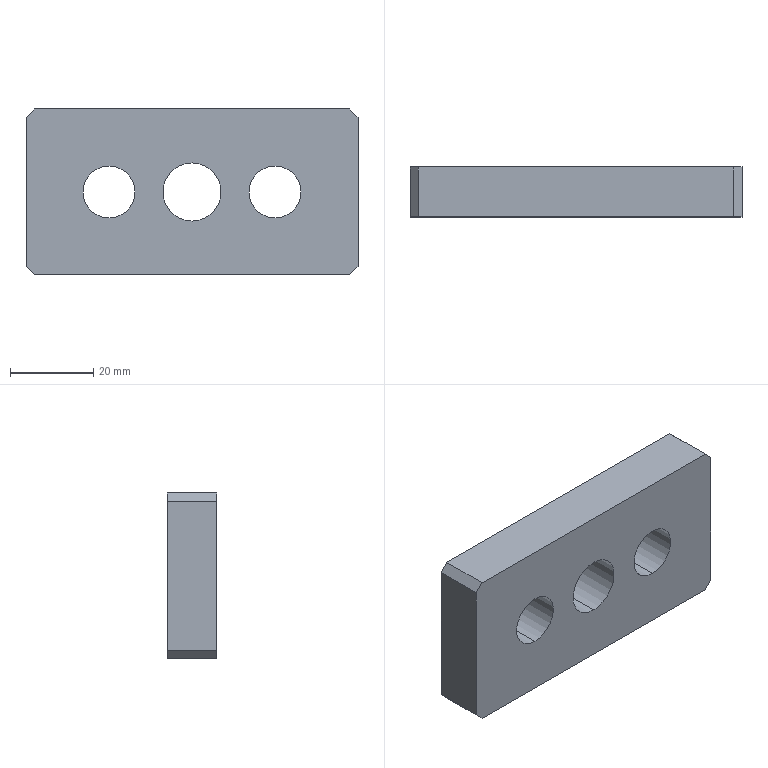Part | STEP file | PN_0026_default | 1 solid | 16 faces | box 80 x 12 x 40 mm | volume 33512 mm3 | plane 10 | cylinder 6 | commonest cylinder face diameters 12.5 x4 14 x2
STEP:
#1=CARTESIAN_POINT('',(0.,0.,0.));
#2=DIRECTION('',(0.,0.,1.));
#3=DIRECTION('',(1.,0.,0.));
#4=AXIS2_PLACEMENT_3D('',#1,#2,#3);
#5=CARTESIAN_POINT('',(-20.,12.,-6.25));
#6=VERTEX_POINT('',#5);
#7=CARTESIAN_POINT('',(-20.,0.,-6.25));
#8=VERTEX_POINT('',#7);
#9=CARTESIAN_POINT('',(-20.,0.,-6.25));
#10=DIRECTION('',(0.,-1.,0.));
#11=VECTOR('',#10,1.);
#12=LINE('',#9,#11);
#13=CARTESIAN_POINT('',(-20.,0.,0.));
#14=DIRECTION('',(0.,-1.,0.));
#15=DIRECTION('',(0.,0.,-1.));
#16=AXIS2_PLACEMENT_3D('',#13,#14,#15);
#17=CYLINDRICAL_SURFACE('',#16,6.25);
#18=CARTESIAN_POINT('',(6.283,0.));
#19=DIRECTION('',(0.,1.));
#20=VECTOR('',#19,1.);
#21=LINE('',#18,#20);
#22=(GEOMETRIC_REPRESENTATION_CONTEXT(2)PARAMETRIC_REPRESENTATION_CONTEXT()REPRESENTATION_CONTEXT('',''));
#23=DEFINITIONAL_REPRESENTATION('',(#21),#22);
#24=PCURVE('',#17,#23);
#25=CARTESIAN_POINT('',(-20.,0.,0.));
#26=DIRECTION('',(0.,-1.,0.));
#27=DIRECTION('',(0.,0.,-1.));
#28=AXIS2_PLACEMENT_3D('',#25,#26,#27);
#29=CYLINDRICAL_SURFACE('',#28,6.25);
#30=CARTESIAN_POINT('',(0.,0.));
#31=DIRECTION('',(0.,1.));
#32=VECTOR('',#31,1.);
#33=LINE('',#30,#32);
#34=(GEOMETRIC_REPRESENTATION_CONTEXT(2)PARAMETRIC_REPRESENTATION_CONTEXT()REPRESENTATION_CONTEXT('',''));
#35=DEFINITIONAL_REPRESENTATION('',(#33),#34);
#36=PCURVE('',#29,#35);
#37=SURFACE_CURVE('',#12,(#24,#36),.PCURVE_S1.);
#38=EDGE_CURVE('',#6,#8,#37,.T.);
#39=ORIENTED_EDGE('',*,*,#38,.T.);
#40=CARTESIAN_POINT('',(-20.,0.,6.25));
#41=VERTEX_POINT('',#40);
#42=CARTESIAN_POINT('',(-20.,0.,0.));
#43=DIRECTION('',(0.,-1.,0.));
#44=DIRECTION('',(0.,0.,-1.));
#45=AXIS2_PLACEMENT_3D('',#42,#43,#44);
#46=CIRCLE('',#45,6.25);
#47=CARTESIAN_POINT('',(0.,0.));
#48=DIRECTION('',(1.,0.));
#49=VECTOR('',#48,1.);
#50=LINE('',#47,#49);
#51=(GEOMETRIC_REPRESENTATION_CONTEXT(2)PARAMETRIC_REPRESENTATION_CONTEXT()REPRESENTATION_CONTEXT('',''));
#52=DEFINITIONAL_REPRESENTATION('',(#50),#51);
#53=PCURVE('',#17,#52);
#54=CARTESIAN_POINT('',(0.,0.,0.));
#55=DIRECTION('',(0.,1.,0.));
#56=DIRECTION('',(0.,0.,1.));
#57=AXIS2_PLACEMENT_3D('',#54,#55,#56);
#58=PLANE('',#57);
#59=CARTESIAN_POINT('',(-6.25,-20.));
#60=CARTESIAN_POINT('',(-6.25,-9.175));
#61=CARTESIAN_POINT('',(3.125,-14.587));
#62=CARTESIAN_POINT('',(12.5,-20.));
#63=CARTESIAN_POINT('',(3.125,-25.413));
#64=CARTESIAN_POINT('',(-6.25,-30.825));
#65=CARTESIAN_POINT('',(-6.25,-20.));
#66=(BOUNDED_CURVE()B_SPLINE_CURVE(2,(#59,#60,#61,#62,#63,#64,#65),.UNSPECIFIED.,.T.,.F.)B_SPLINE_CURVE_WITH_KNOTS((1,2,2,2,2,1),(-2.094,0.,2.094,4.189,6.283,8.378),.UNSPECIFIED.)CURVE()GEOMETRIC_REPRESENTATION_ITEM()RATIONAL_B_SPLINE_CURVE((1.,0.5,1.,0.5,1.,0.5,1.))REPRESENTATION_ITEM(''));
#67=(GEOMETRIC_REPRESENTATION_CONTEXT(2)PARAMETRIC_REPRESENTATION_CONTEXT()REPRESENTATION_CONTEXT('',''));
#68=DEFINITIONAL_REPRESENTATION('',(#66),#67);
#69=PCURVE('',#58,#68);
#70=SURFACE_CURVE('',#46,(#53,#69),.PCURVE_S1.);
#71=EDGE_CURVE('',#41,#8,#70,.T.);
#72=ORIENTED_EDGE('',*,*,#71,.F.);
#73=CARTESIAN_POINT('',(-20.,12.,6.25));
#74=VERTEX_POINT('',#73);
#75=CARTESIAN_POINT('',(-20.,0.,6.25));
#76=DIRECTION('',(0.,-1.,0.));
#77=VECTOR('',#76,1.);
#78=LINE('',#75,#77);
#79=CARTESIAN_POINT('',(3.142,0.));
#80=DIRECTION('',(0.,1.));
#81=VECTOR('',#80,1.);
#82=LINE('',#79,#81);
#83=(GEOMETRIC_REPRESENTATION_CONTEXT(2)PARAMETRIC_REPRESENTATION_CONTEXT()REPRESENTATION_CONTEXT('',''));
#84=DEFINITIONAL_REPRESENTATION('',(#82),#83);
#85=PCURVE('',#17,#84);
#86=CARTESIAN_POINT('',(3.142,0.));
#87=DIRECTION('',(0.,1.));
#88=VECTOR('',#87,1.);
#89=LINE('',#86,#88);
#90=(GEOMETRIC_REPRESENTATION_CONTEXT(2)PARAMETRIC_REPRESENTATION_CONTEXT()REPRESENTATION_CONTEXT('',''));
#91=DEFINITIONAL_REPRESENTATION('',(#89),#90);
#92=PCURVE('',#29,#91);
#93=SURFACE_CURVE('',#78,(#85,#92),.PCURVE_S1.);
#94=EDGE_CURVE('',#74,#41,#93,.T.);
#95=ORIENTED_EDGE('',*,*,#94,.F.);
#96=CARTESIAN_POINT('',(-20.,12.,0.));
#97=DIRECTION('',(0.,-1.,0.));
#98=DIRECTION('',(0.,0.,-1.));
#99=AXIS2_PLACEMENT_3D('',#96,#97,#98);
#100=CIRCLE('',#99,6.25);
#101=CARTESIAN_POINT('',(0.,-12.));
#102=DIRECTION('',(1.,0.));
#103=VECTOR('',#102,1.);
#104=LINE('',#101,#103);
#105=(GEOMETRIC_REPRESENTATION_CONTEXT(2)PARAMETRIC_REPRESENTATION_CONTEXT()REPRESENTATION_CONTEXT('',''));
#106=DEFINITIONAL_REPRESENTATION('',(#104),#105);
#107=PCURVE('',#17,#106);
#108=CARTESIAN_POINT('',(0.,12.,0.));
#109=DIRECTION('',(0.,1.,0.));
#110=DIRECTION('',(0.,0.,1.));
#111=AXIS2_PLACEMENT_3D('',#108,#109,#110);
#112=PLANE('',#111);
#113=CARTESIAN_POINT('',(-6.25,-20.));
#114=CARTESIAN_POINT('',(-6.25,-9.175));
#115=CARTESIAN_POINT('',(3.125,-14.587));
#116=CARTESIAN_POINT('',(12.5,-20.));
#117=CARTESIAN_POINT('',(3.125,-25.413));
#118=CARTESIAN_POINT('',(-6.25,-30.825));
#119=CARTESIAN_POINT('',(-6.25,-20.));
#120=(BOUNDED_CURVE()B_SPLINE_CURVE(2,(#113,#114,#115,#116,#117,#118,#119),.UNSPECIFIED.,.T.,.F.)B_SPLINE_CURVE_WITH_KNOTS((1,2,2,2,2,1),(-2.094,0.,2.094,4.189,6.283,8.378),.UNSPECIFIED.)CURVE()GEOMETRIC_REPRESENTATION_ITEM()RATIONAL_B_SPLINE_CURVE((1.,0.5,1.,0.5,1.,0.5,1.))REPRESENTATION_ITEM(''));
#121=(GEOMETRIC_REPRESENTATION_CONTEXT(2)PARAMETRIC_REPRESENTATION_CONTEXT()REPRESENTATION_CONTEXT('',''));
#122=DEFINITIONAL_REPRESENTATION('',(#120),#121);
#123=PCURVE('',#112,#122);
#124=SURFACE_CURVE('',#100,(#107,#123),.PCURVE_S1.);
#125=EDGE_CURVE('',#74,#6,#124,.T.);
#126=ORIENTED_EDGE('',*,*,#125,.T.);
#127=EDGE_LOOP('',(#39,#72,#95,#126));
#128=FACE_BOUND('',#127,.F.);
#129=ADVANCED_FACE('',(#128),#17,.F.);
#130=CARTESIAN_POINT('',(20.,12.,-6.25));
#131=VERTEX_POINT('',#130);
#132=CARTESIAN_POINT('',(20.,0.,-6.25));
#133=VERTEX_POINT('',#132);
#134=CARTESIAN_POINT('',(20.,0.,-6.25));
#135=DIRECTION('',(0.,-1.,0.));
#136=VECTOR('',#135,1.);
#137=LINE('',#134,#136);
#138=CARTESIAN_POINT('',(20.,0.,0.));
#139=DIRECTION('',(0.,-1.,0.));
#140=DIRECTION('',(0.,0.,-1.));
#141=AXIS2_PLACEMENT_3D('',#138,#139,#140);
#142=CYLINDRICAL_SURFACE('',#141,6.25);
#143=CARTESIAN_POINT('',(6.283,0.));
#144=DIRECTION('',(0.,1.));
#145=VECTOR('',#144,1.);
#146=LINE('',#143,#145);
#147=(GEOMETRIC_REPRESENTATION_CONTEXT(2)PARAMETRIC_REPRESENTATION_CONTEXT()REPRESENTATION_CONTEXT('',''));
#148=DEFINITIONAL_REPRESENTATION('',(#146),#147);
#149=PCURVE('',#142,#148);
#150=CARTESIAN_POINT('',(20.,0.,0.));
#151=DIRECTION('',(0.,-1.,0.));
#152=DIRECTION('',(0.,0.,-1.));
#153=AXIS2_PLACEMENT_3D('',#150,#151,#152);
#154=CYLINDRICAL_SURFACE('',#153,6.25);
#155=CARTESIAN_POINT('',(0.,0.));
#156=DIRECTION('',(0.,1.));
#157=VECTOR('',#156,1.);
#158=LINE('',#155,#157);
#159=(GEOMETRIC_REPRESENTATION_CONTEXT(2)PARAMETRIC_REPRESENTATION_CONTEXT()REPRESENTATION_CONTEXT('',''));
#160=DEFINITIONAL_REPRESENTATION('',(#158),#159);
#161=PCURVE('',#154,#160);
#162=SURFACE_CURVE('',#137,(#149,#161),.PCURVE_S1.);
#163=EDGE_CURVE('',#131,#133,#162,.T.);
#164=ORIENTED_EDGE('',*,*,#163,.T.);
#165=CARTESIAN_POINT('',(20.,0.,6.25));
#166=VERTEX_POINT('',#165);
#167=CARTESIAN_POINT('',(20.,0.,0.));
#168=DIRECTION('',(0.,-1.,0.));
#169=DIRECTION('',(0.,0.,-1.));
#170=AXIS2_PLACEMENT_3D('',#167,#168,#169);
#171=CIRCLE('',#170,6.25);
#172=CARTESIAN_POINT('',(0.,0.));
#173=DIRECTION('',(1.,0.));
#174=VECTOR('',#173,1.);
#175=LINE('',#172,#174);
#176=(GEOMETRIC_REPRESENTATION_CONTEXT(2)PARAMETRIC_REPRESENTATION_CONTEXT()REPRESENTATION_CONTEXT('',''));
#177=DEFINITIONAL_REPRESENTATION('',(#175),#176);
#178=PCURVE('',#142,#177);
#179=CARTESIAN_POINT('',(-6.25,20.));
#180=CARTESIAN_POINT('',(-6.25,30.825));
#181=CARTESIAN_POINT('',(3.125,25.413));
#182=CARTESIAN_POINT('',(12.5,20.));
#183=CARTESIAN_POINT('',(3.125,14.587));
#184=CARTESIAN_POINT('',(-6.25,9.175));
#185=CARTESIAN_POINT('',(-6.25,20.));
#186=(BOUNDED_CURVE()B_SPLINE_CURVE(2,(#179,#180,#181,#182,#183,#184,#185),.UNSPECIFIED.,.T.,.F.)B_SPLINE_CURVE_WITH_KNOTS((1,2,2,2,2,1),(-2.094,0.,2.094,4.189,6.283,8.378),.UNSPECIFIED.)CURVE()GEOMETRIC_REPRESENTATION_ITEM()RATIONAL_B_SPLINE_CURVE((1.,0.5,1.,0.5,1.,0.5,1.))REPRESENTATION_ITEM(''));
#187=(GEOMETRIC_REPRESENTATION_CONTEXT(2)PARAMETRIC_REPRESENTATION_CONTEXT()REPRESENTATION_CONTEXT('',''));
#188=DEFINITIONAL_REPRESENTATION('',(#186),#187);
#189=PCURVE('',#58,#188);
#190=SURFACE_CURVE('',#171,(#178,#189),.PCURVE_S1.);
#191=EDGE_CURVE('',#166,#133,#190,.T.);
#192=ORIENTED_EDGE('',*,*,#191,.F.);
#193=CARTESIAN_POINT('',(20.,12.,6.25));
#194=VERTEX_POINT('',#193);
#195=CARTESIAN_POINT('',(20.,0.,6.25));
#196=DIRECTION('',(0.,-1.,0.));
#197=VECTOR('',#196,1.);
#198=LINE('',#195,#197);
#199=CARTESIAN_POINT('',(3.142,0.));
#200=DIRECTION('',(0.,1.));
#201=VECTOR('',#200,1.);
#202=LINE('',#199,#201);
#203=(GEOMETRIC_REPRESENTATION_CONTEXT(2)PARAMETRIC_REPRESENTATION_CONTEXT()REPRESENTATION_CONTEXT('',''));
#204=DEFINITIONAL_REPRESENTATION('',(#202),#203);
#205=PCURVE('',#142,#204);
#206=CARTESIAN_POINT('',(3.142,0.));
#207=DIRECTION('',(0.,1.));
#208=VECTOR('',#207,1.);
#209=LINE('',#206,#208);
#210=(GEOMETRIC_REPRESENTATION_CONTEXT(2)PARAMETRIC_REPRESENTATION_CONTEXT()REPRESENTATION_CONTEXT('',''));
#211=DEFINITIONAL_REPRESENTATION('',(#209),#210);
#212=PCURVE('',#154,#211);
#213=SURFACE_CURVE('',#198,(#205,#212),.PCURVE_S1.);
#214=EDGE_CURVE('',#194,#166,#213,.T.);
#215=ORIENTED_EDGE('',*,*,#214,.F.);
#216=CARTESIAN_POINT('',(20.,12.,0.));
#217=DIRECTION('',(0.,-1.,0.));
#218=DIRECTION('',(0.,0.,-1.));
#219=AXIS2_PLACEMENT_3D('',#216,#217,#218);
#220=CIRCLE('',#219,6.25);
#221=CARTESIAN_POINT('',(0.,-12.));
#222=DIRECTION('',(1.,0.));
#223=VECTOR('',#222,1.);
#224=LINE('',#221,#223);
#225=(GEOMETRIC_REPRESENTATION_CONTEXT(2)PARAMETRIC_REPRESENTATION_CONTEXT()REPRESENTATION_CONTEXT('',''));
#226=DEFINITIONAL_REPRESENTATION('',(#224),#225);
#227=PCURVE('',#142,#226);
#228=CARTESIAN_POINT('',(-6.25,20.));
#229=CARTESIAN_POINT('',(-6.25,30.825));
#230=CARTESIAN_POINT('',(3.125,25.413));
#231=CARTESIAN_POINT('',(12.5,20.));
#232=CARTESIAN_POINT('',(3.125,14.587));
#233=CARTESIAN_POINT('',(-6.25,9.175));
#234=CARTESIAN_POINT('',(-6.25,20.));
#235=(BOUNDED_CURVE()B_SPLINE_CURVE(2,(#228,#229,#230,#231,#232,#233,#234),.UNSPECIFIED.,.T.,.F.)B_SPLINE_CURVE_WITH_KNOTS((1,2,2,2,2,1),(-2.094,0.,2.094,4.189,6.283,8.378),.UNSPECIFIED.)CURVE()GEOMETRIC_REPRESENTATION_ITEM()RATIONAL_B_SPLINE_CURVE((1.,0.5,1.,0.5,1.,0.5,1.))REPRESENTATION_ITEM(''));
#236=(GEOMETRIC_REPRESENTATION_CONTEXT(2)PARAMETRIC_REPRESENTATION_CONTEXT()REPRESENTATION_CONTEXT('',''));
#237=DEFINITIONAL_REPRESENTATION('',(#235),#236);
#238=PCURVE('',#112,#237);
#239=SURFACE_CURVE('',#220,(#227,#238),.PCURVE_S1.);
#240=EDGE_CURVE('',#194,#131,#239,.T.);
#241=ORIENTED_EDGE('',*,*,#240,.T.);
#242=EDGE_LOOP('',(#164,#192,#215,#241));
#243=FACE_BOUND('',#242,.F.);
#244=ADVANCED_FACE('',(#243),#142,.F.);
#245=CARTESIAN_POINT('',(0.,12.,-7.));
#246=VERTEX_POINT('',#245);
#247=CARTESIAN_POINT('',(0.,0.,-7.));
#248=VERTEX_POINT('',#247);
#249=CARTESIAN_POINT('',(0.,0.,-7.));
#250=DIRECTION('',(0.,-1.,0.));
#251=VECTOR('',#250,1.);
#252=LINE('',#249,#251);
#253=CARTESIAN_POINT('',(0.,0.,0.));
#254=DIRECTION('',(0.,-1.,0.));
#255=DIRECTION('',(0.,0.,-1.));
#256=AXIS2_PLACEMENT_3D('',#253,#254,#255);
#257=CYLINDRICAL_SURFACE('',#256,7.);
#258=CARTESIAN_POINT('',(6.283,0.));
#259=DIRECTION('',(0.,1.));
#260=VECTOR('',#259,1.);
#261=LINE('',#258,#260);
#262=(GEOMETRIC_REPRESENTATION_CONTEXT(2)PARAMETRIC_REPRESENTATION_CONTEXT()REPRESENTATION_CONTEXT('',''));
#263=DEFINITIONAL_REPRESENTATION('',(#261),#262);
#264=PCURVE('',#257,#263);
#265=CARTESIAN_POINT('',(0.,0.,0.));
#266=DIRECTION('',(0.,-1.,0.));
#267=DIRECTION('',(0.,0.,-1.));
#268=AXIS2_PLACEMENT_3D('',#265,#266,#267);
#269=CYLINDRICAL_SURFACE('',#268,7.);
#270=CARTESIAN_POINT('',(0.,0.));
#271=DIRECTION('',(0.,1.));
#272=VECTOR('',#271,1.);
#273=LINE('',#270,#272);
#274=(GEOMETRIC_REPRESENTATION_CONTEXT(2)PARAMETRIC_REPRESENTATION_CONTEXT()REPRESENTATION_CONTEXT('',''));
#275=DEFINITIONAL_REPRESENTATION('',(#273),#274);
#276=PCURVE('',#269,#275);
#277=SURFACE_CURVE('',#252,(#264,#276),.PCURVE_S1.);
#278=EDGE_CURVE('',#246,#248,#277,.T.);
#279=ORIENTED_EDGE('',*,*,#278,.T.);
#280=CARTESIAN_POINT('',(0.,0.,7.));
#281=VERTEX_POINT('',#280);
#282=CARTESIAN_POINT('',(0.,0.,0.));
#283=DIRECTION('',(0.,-1.,0.));
#284=DIRECTION('',(0.,0.,-1.));
#285=AXIS2_PLACEMENT_3D('',#282,#283,#284);
#286=CIRCLE('',#285,7.);
#287=CARTESIAN_POINT('',(0.,0.));
#288=DIRECTION('',(1.,0.));
#289=VECTOR('',#288,1.);
#290=LINE('',#287,#289);
#291=(GEOMETRIC_REPRESENTATION_CONTEXT(2)PARAMETRIC_REPRESENTATION_CONTEXT()REPRESENTATION_CONTEXT('',''));
#292=DEFINITIONAL_REPRESENTATION('',(#290),#291);
#293=PCURVE('',#257,#292);
#294=CARTESIAN_POINT('',(-7.,0.));
#295=CARTESIAN_POINT('',(-7.,12.124));
#296=CARTESIAN_POINT('',(3.5,6.062));
#297=CARTESIAN_POINT('',(14.,0.));
#298=CARTESIAN_POINT('',(3.5,-6.062));
#299=CARTESIAN_POINT('',(-7.,-12.124));
#300=CARTESIAN_POINT('',(-7.,0.));
#301=(BOUNDED_CURVE()B_SPLINE_CURVE(2,(#294,#295,#296,#297,#298,#299,#300),.UNSPECIFIED.,.T.,.F.)B_SPLINE_CURVE_WITH_KNOTS((1,2,2,2,2,1),(-2.094,0.,2.094,4.189,6.283,8.378),.UNSPECIFIED.)CURVE()GEOMETRIC_REPRESENTATION_ITEM()RATIONAL_B_SPLINE_CURVE((1.,0.5,1.,0.5,1.,0.5,1.))REPRESENTATION_ITEM(''));
#302=(GEOMETRIC_REPRESENTATION_CONTEXT(2)PARAMETRIC_REPRESENTATION_CONTEXT()REPRESENTATION_CONTEXT('',''));
#303=DEFINITIONAL_REPRESENTATION('',(#301),#302);
#304=PCURVE('',#58,#303);
#305=SURFACE_CURVE('',#286,(#293,#304),.PCURVE_S1.);
#306=EDGE_CURVE('',#281,#248,#305,.T.);
#307=ORIENTED_EDGE('',*,*,#306,.F.);
#308=CARTESIAN_POINT('',(0.,12.,7.));
#309=VERTEX_POINT('',#308);
#310=CARTESIAN_POINT('',(0.,0.,7.));
#311=DIRECTION('',(0.,-1.,0.));
#312=VECTOR('',#311,1.);
#313=LINE('',#310,#312);
#314=CARTESIAN_POINT('',(3.142,0.));
#315=DIRECTION('',(0.,1.));
#316=VECTOR('',#315,1.);
#317=LINE('',#314,#316);
#318=(GEOMETRIC_REPRESENTATION_CONTEXT(2)PARAMETRIC_REPRESENTATION_CONTEXT()REPRESENTATION_CONTEXT('',''));
#319=DEFINITIONAL_REPRESENTATION('',(#317),#318);
#320=PCURVE('',#257,#319);
#321=CARTESIAN_POINT('',(3.142,0.));
#322=DIRECTION('',(0.,1.));
#323=VECTOR('',#322,1.);
#324=LINE('',#321,#323);
#325=(GEOMETRIC_REPRESENTATION_CONTEXT(2)PARAMETRIC_REPRESENTATION_CONTEXT()REPRESENTATION_CONTEXT('',''));
#326=DEFINITIONAL_REPRESENTATION('',(#324),#325);
#327=PCURVE('',#269,#326);
#328=SURFACE_CURVE('',#313,(#320,#327),.PCURVE_S1.);
#329=EDGE_CURVE('',#309,#281,#328,.T.);
#330=ORIENTED_EDGE('',*,*,#329,.F.);
#331=CARTESIAN_POINT('',(0.,12.,0.));
#332=DIRECTION('',(0.,1.,0.));
#333=DIRECTION('',(0.,0.,1.));
#334=AXIS2_PLACEMENT_3D('',#331,#332,#333);
#335=CIRCLE('',#334,7.);
#336=CARTESIAN_POINT('',(9.425,-12.));
#337=DIRECTION('',(-1.,0.));
#338=VECTOR('',#337,1.);
#339=LINE('',#336,#338);
#340=(GEOMETRIC_REPRESENTATION_CONTEXT(2)PARAMETRIC_REPRESENTATION_CONTEXT()REPRESENTATION_CONTEXT('',''));
#341=DEFINITIONAL_REPRESENTATION('',(#339),#340);
#342=PCURVE('',#257,#341);
#343=CARTESIAN_POINT('',(0.,0.));
#344=DIRECTION('',(1.,0.));
#345=AXIS2_PLACEMENT_2D('',#343,#344);
#346=CIRCLE('',#345,7.);
#347=(GEOMETRIC_REPRESENTATION_CONTEXT(2)PARAMETRIC_REPRESENTATION_CONTEXT()REPRESENTATION_CONTEXT('',''));
#348=DEFINITIONAL_REPRESENTATION('',(#346),#347);
#349=PCURVE('',#112,#348);
#350=SURFACE_CURVE('',#335,(#342,#349),.PCURVE_S1.);
#351=EDGE_CURVE('',#246,#309,#350,.T.);
#352=ORIENTED_EDGE('',*,*,#351,.F.);
#353=EDGE_LOOP('',(#279,#307,#330,#352));
#354=FACE_BOUND('',#353,.F.);
#355=ADVANCED_FACE('',(#354),#257,.F.);
#356=CARTESIAN_POINT('',(40.,0.,18.));
#357=VERTEX_POINT('',#356);
#358=CARTESIAN_POINT('',(40.,0.,-18.));
#359=VERTEX_POINT('',#358);
#360=CARTESIAN_POINT('',(40.,0.,-20.));
#361=DIRECTION('',(0.,0.,-1.));
#362=VECTOR('',#361,1.);
#363=LINE('',#360,#362);
#364=CARTESIAN_POINT('',(40.,12.,-20.));
#365=DIRECTION('',(-1.,0.,0.));
#366=DIRECTION('',(0.,0.,1.));
#367=AXIS2_PLACEMENT_3D('',#364,#365,#366);
#368=PLANE('',#367);
#369=CARTESIAN_POINT('',(0.,-12.));
#370=DIRECTION('',(-1.,0.));
#371=VECTOR('',#370,1.);
#372=LINE('',#369,#371);
#373=(GEOMETRIC_REPRESENTATION_CONTEXT(2)PARAMETRIC_REPRESENTATION_CONTEXT()REPRESENTATION_CONTEXT('',''));
#374=DEFINITIONAL_REPRESENTATION('',(#372),#373);
#375=PCURVE('',#368,#374);
#376=CARTESIAN_POINT('',(-20.,40.));
#377=DIRECTION('',(-1.,0.));
#378=VECTOR('',#377,1.);
#379=LINE('',#376,#378);
#380=(GEOMETRIC_REPRESENTATION_CONTEXT(2)PARAMETRIC_REPRESENTATION_CONTEXT()REPRESENTATION_CONTEXT('',''));
#381=DEFINITIONAL_REPRESENTATION('',(#379),#380);
#382=PCURVE('',#58,#381);
#383=SURFACE_CURVE('',#363,(#375,#382),.PCURVE_S1.);
#384=EDGE_CURVE('',#357,#359,#383,.T.);
#385=ORIENTED_EDGE('',*,*,#384,.T.);
#386=CARTESIAN_POINT('',(40.,12.,-18.));
#387=VERTEX_POINT('',#386);
#388=CARTESIAN_POINT('',(40.,12.,-18.));
#389=DIRECTION('',(0.,1.,0.));
#390=VECTOR('',#389,1.);
#391=LINE('',#388,#390);
#392=CARTESIAN_POINT('',(2.,0.));
#393=DIRECTION('',(0.,1.));
#394=VECTOR('',#393,1.);
#395=LINE('',#392,#394);
#396=(GEOMETRIC_REPRESENTATION_CONTEXT(2)PARAMETRIC_REPRESENTATION_CONTEXT()REPRESENTATION_CONTEXT('',''));
#397=DEFINITIONAL_REPRESENTATION('',(#395),#396);
#398=PCURVE('',#368,#397);
#399=CARTESIAN_POINT('',(38.,12.,-20.));
#400=DIRECTION('',(-0.7071,0.,0.7071));
#401=DIRECTION('',(0.,-1.,0.));
#402=AXIS2_PLACEMENT_3D('',#399,#400,#401);
#403=PLANE('',#402);
#404=CARTESIAN_POINT('',(0.,2.828));
#405=DIRECTION('',(-1.,0.));
#406=VECTOR('',#405,1.);
#407=LINE('',#404,#406);
#408=(GEOMETRIC_REPRESENTATION_CONTEXT(2)PARAMETRIC_REPRESENTATION_CONTEXT()REPRESENTATION_CONTEXT('',''));
#409=DEFINITIONAL_REPRESENTATION('',(#407),#408);
#410=PCURVE('',#403,#409);
#411=SURFACE_CURVE('',#391,(#398,#410),.PCURVE_S1.);
#412=EDGE_CURVE('',#359,#387,#411,.T.);
#413=ORIENTED_EDGE('',*,*,#412,.T.);
#414=CARTESIAN_POINT('',(40.,12.,18.));
#415=VERTEX_POINT('',#414);
#416=CARTESIAN_POINT('',(40.,12.,-20.));
#417=DIRECTION('',(0.,0.,-1.));
#418=VECTOR('',#417,1.);
#419=LINE('',#416,#418);
#420=CARTESIAN_POINT('',(0.,0.));
#421=DIRECTION('',(-1.,0.));
#422=VECTOR('',#421,1.);
#423=LINE('',#420,#422);
#424=(GEOMETRIC_REPRESENTATION_CONTEXT(2)PARAMETRIC_REPRESENTATION_CONTEXT()REPRESENTATION_CONTEXT('',''));
#425=DEFINITIONAL_REPRESENTATION('',(#423),#424);
#426=PCURVE('',#368,#425);
#427=CARTESIAN_POINT('',(-20.,40.));
#428=DIRECTION('',(-1.,0.));
#429=VECTOR('',#428,1.);
#430=LINE('',#427,#429);
#431=(GEOMETRIC_REPRESENTATION_CONTEXT(2)PARAMETRIC_REPRESENTATION_CONTEXT()REPRESENTATION_CONTEXT('',''));
#432=DEFINITIONAL_REPRESENTATION('',(#430),#431);
#433=PCURVE('',#112,#432);
#434=SURFACE_CURVE('',#419,(#426,#433),.PCURVE_S1.);
#435=EDGE_CURVE('',#415,#387,#434,.T.);
#436=ORIENTED_EDGE('',*,*,#435,.F.);
#437=CARTESIAN_POINT('',(40.,12.,18.));
#438=DIRECTION('',(0.,-1.,0.));
#439=VECTOR('',#438,1.);
#440=LINE('',#437,#439);
#441=CARTESIAN_POINT('',(38.,0.));
#442=DIRECTION('',(0.,-1.));
#443=VECTOR('',#442,1.);
#444=LINE('',#441,#443);
#445=(GEOMETRIC_REPRESENTATION_CONTEXT(2)PARAMETRIC_REPRESENTATION_CONTEXT()REPRESENTATION_CONTEXT('',''));
#446=DEFINITIONAL_REPRESENTATION('',(#444),#445);
#447=PCURVE('',#368,#446);
#448=CARTESIAN_POINT('',(40.,12.,18.));
#449=DIRECTION('',(-0.7071,0.,-0.7071));
#450=DIRECTION('',(0.,-1.,0.));
#451=AXIS2_PLACEMENT_3D('',#448,#449,#450);
#452=PLANE('',#451);
#453=CARTESIAN_POINT('',(0.,0.));
#454=DIRECTION('',(1.,0.));
#455=VECTOR('',#454,1.);
#456=LINE('',#453,#455);
#457=(GEOMETRIC_REPRESENTATION_CONTEXT(2)PARAMETRIC_REPRESENTATION_CONTEXT()REPRESENTATION_CONTEXT('',''));
#458=DEFINITIONAL_REPRESENTATION('',(#456),#457);
#459=PCURVE('',#452,#458);
#460=SURFACE_CURVE('',#440,(#447,#459),.PCURVE_S1.);
#461=EDGE_CURVE('',#415,#357,#460,.T.);
#462=ORIENTED_EDGE('',*,*,#461,.T.);
#463=EDGE_LOOP('',(#385,#413,#436,#462));
#464=FACE_BOUND('',#463,.T.);
#465=ADVANCED_FACE('',(#464),#368,.F.);
#466=CARTESIAN_POINT('',(38.,0.,-20.));
#467=VERTEX_POINT('',#466);
#468=CARTESIAN_POINT('',(-38.,0.,-20.));
#469=VERTEX_POINT('',#468);
#470=CARTESIAN_POINT('',(-40.,0.,-20.));
#471=DIRECTION('',(-1.,0.,0.));
#472=VECTOR('',#471,1.);
#473=LINE('',#470,#472);
#474=CARTESIAN_POINT('',(-40.,12.,-20.));
#475=DIRECTION('',(0.,0.,1.));
#476=DIRECTION('',(1.,0.,0.));
#477=AXIS2_PLACEMENT_3D('',#474,#475,#476);
#478=PLANE('',#477);
#479=CARTESIAN_POINT('',(0.,-12.));
#480=DIRECTION('',(-1.,0.));
#481=VECTOR('',#480,1.);
#482=LINE('',#479,#481);
#483=(GEOMETRIC_REPRESENTATION_CONTEXT(2)PARAMETRIC_REPRESENTATION_CONTEXT()REPRESENTATION_CONTEXT('',''));
#484=DEFINITIONAL_REPRESENTATION('',(#482),#483);
#485=PCURVE('',#478,#484);
#486=CARTESIAN_POINT('',(-20.,-40.));
#487=DIRECTION('',(0.,-1.));
#488=VECTOR('',#487,1.);
#489=LINE('',#486,#488);
#490=(GEOMETRIC_REPRESENTATION_CONTEXT(2)PARAMETRIC_REPRESENTATION_CONTEXT()REPRESENTATION_CONTEXT('',''));
#491=DEFINITIONAL_REPRESENTATION('',(#489),#490);
#492=PCURVE('',#58,#491);
#493=SURFACE_CURVE('',#473,(#485,#492),.PCURVE_S1.);
#494=EDGE_CURVE('',#467,#469,#493,.T.);
#495=ORIENTED_EDGE('',*,*,#494,.T.);
#496=CARTESIAN_POINT('',(-38.,12.,-20.));
#497=VERTEX_POINT('',#496);
#498=CARTESIAN_POINT('',(-38.,12.,-20.));
#499=DIRECTION('',(0.,1.,0.));
#500=VECTOR('',#499,1.);
#501=LINE('',#498,#500);
#502=CARTESIAN_POINT('',(2.,0.));
#503=DIRECTION('',(0.,1.));
#504=VECTOR('',#503,1.);
#505=LINE('',#502,#504);
#506=(GEOMETRIC_REPRESENTATION_CONTEXT(2)PARAMETRIC_REPRESENTATION_CONTEXT()REPRESENTATION_CONTEXT('',''));
#507=DEFINITIONAL_REPRESENTATION('',(#505),#506);
#508=PCURVE('',#478,#507);
#509=CARTESIAN_POINT('',(-40.,12.,-18.));
#510=DIRECTION('',(0.7071,0.,0.7071));
#511=DIRECTION('',(0.,-1.,0.));
#512=AXIS2_PLACEMENT_3D('',#509,#510,#511);
#513=PLANE('',#512);
#514=CARTESIAN_POINT('',(0.,2.828));
#515=DIRECTION('',(-1.,0.));
#516=VECTOR('',#515,1.);
#517=LINE('',#514,#516);
#518=(GEOMETRIC_REPRESENTATION_CONTEXT(2)PARAMETRIC_REPRESENTATION_CONTEXT()REPRESENTATION_CONTEXT('',''));
#519=DEFINITIONAL_REPRESENTATION('',(#517),#518);
#520=PCURVE('',#513,#519);
#521=SURFACE_CURVE('',#501,(#508,#520),.PCURVE_S1.);
#522=EDGE_CURVE('',#469,#497,#521,.T.);
#523=ORIENTED_EDGE('',*,*,#522,.T.);
#524=CARTESIAN_POINT('',(38.,12.,-20.));
#525=VERTEX_POINT('',#524);
#526=CARTESIAN_POINT('',(-40.,12.,-20.));
#527=DIRECTION('',(-1.,0.,0.));
#528=VECTOR('',#527,1.);
#529=LINE('',#526,#528);
#530=CARTESIAN_POINT('',(0.,0.));
#531=DIRECTION('',(-1.,0.));
#532=VECTOR('',#531,1.);
#533=LINE('',#530,#532);
#534=(GEOMETRIC_REPRESENTATION_CONTEXT(2)PARAMETRIC_REPRESENTATION_CONTEXT()REPRESENTATION_CONTEXT('',''));
#535=DEFINITIONAL_REPRESENTATION('',(#533),#534);
#536=PCURVE('',#478,#535);
#537=CARTESIAN_POINT('',(-20.,-40.));
#538=DIRECTION('',(0.,-1.));
#539=VECTOR('',#538,1.);
#540=LINE('',#537,#539);
#541=(GEOMETRIC_REPRESENTATION_CONTEXT(2)PARAMETRIC_REPRESENTATION_CONTEXT()REPRESENTATION_CONTEXT('',''));
#542=DEFINITIONAL_REPRESENTATION('',(#540),#541);
#543=PCURVE('',#112,#542);
#544=SURFACE_CURVE('',#529,(#536,#543),.PCURVE_S1.);
#545=EDGE_CURVE('',#525,#497,#544,.T.);
#546=ORIENTED_EDGE('',*,*,#545,.F.);
#547=CARTESIAN_POINT('',(38.,12.,-20.));
#548=DIRECTION('',(0.,-1.,0.));
#549=VECTOR('',#548,1.);
#550=LINE('',#547,#549);
#551=CARTESIAN_POINT('',(78.,0.));
#552=DIRECTION('',(0.,-1.));
#553=VECTOR('',#552,1.);
#554=LINE('',#551,#553);
#555=(GEOMETRIC_REPRESENTATION_CONTEXT(2)PARAMETRIC_REPRESENTATION_CONTEXT()REPRESENTATION_CONTEXT('',''));
#556=DEFINITIONAL_REPRESENTATION('',(#554),#555);
#557=PCURVE('',#478,#556);
#558=CARTESIAN_POINT('',(0.,0.));
#559=DIRECTION('',(1.,0.));
#560=VECTOR('',#559,1.);
#561=LINE('',#558,#560);
#562=(GEOMETRIC_REPRESENTATION_CONTEXT(2)PARAMETRIC_REPRESENTATION_CONTEXT()REPRESENTATION_CONTEXT('',''));
#563=DEFINITIONAL_REPRESENTATION('',(#561),#562);
#564=PCURVE('',#403,#563);
#565=SURFACE_CURVE('',#550,(#557,#564),.PCURVE_S1.);
#566=EDGE_CURVE('',#525,#467,#565,.T.);
#567=ORIENTED_EDGE('',*,*,#566,.T.);
#568=EDGE_LOOP('',(#495,#523,#546,#567));
#569=FACE_BOUND('',#568,.T.);
#570=ADVANCED_FACE('',(#569),#478,.F.);
#571=CARTESIAN_POINT('',(-40.,12.,-18.));
#572=VERTEX_POINT('',#571);
#573=CARTESIAN_POINT('',(-40.,12.,18.));
#574=VERTEX_POINT('',#573);
#575=CARTESIAN_POINT('',(-40.,12.,-20.));
#576=DIRECTION('',(0.,0.,1.));
#577=VECTOR('',#576,1.);
#578=LINE('',#575,#577);
#579=CARTESIAN_POINT('',(-40.,12.,-20.));
#580=DIRECTION('',(1.,0.,0.));
#581=DIRECTION('',(0.,0.,-1.));
#582=AXIS2_PLACEMENT_3D('',#579,#580,#581);
#583=PLANE('',#582);
#584=CARTESIAN_POINT('',(0.,0.));
#585=DIRECTION('',(-1.,0.));
#586=VECTOR('',#585,1.);
#587=LINE('',#584,#586);
#588=(GEOMETRIC_REPRESENTATION_CONTEXT(2)PARAMETRIC_REPRESENTATION_CONTEXT()REPRESENTATION_CONTEXT('',''));
#589=DEFINITIONAL_REPRESENTATION('',(#587),#588);
#590=PCURVE('',#583,#589);
#591=CARTESIAN_POINT('',(-20.,-40.));
#592=DIRECTION('',(1.,0.));
#593=VECTOR('',#592,1.);
#594=LINE('',#591,#593);
#595=(GEOMETRIC_REPRESENTATION_CONTEXT(2)PARAMETRIC_REPRESENTATION_CONTEXT()REPRESENTATION_CONTEXT('',''));
#596=DEFINITIONAL_REPRESENTATION('',(#594),#595);
#597=PCURVE('',#112,#596);
#598=SURFACE_CURVE('',#578,(#590,#597),.PCURVE_S1.);
#599=EDGE_CURVE('',#572,#574,#598,.T.);
#600=ORIENTED_EDGE('',*,*,#599,.F.);
#601=CARTESIAN_POINT('',(-40.,0.,-18.));
#602=VERTEX_POINT('',#601);
#603=CARTESIAN_POINT('',(-40.,12.,-18.));
#604=DIRECTION('',(0.,-1.,0.));
#605=VECTOR('',#604,1.);
#606=LINE('',#603,#605);
#607=CARTESIAN_POINT('',(-2.,0.));
#608=DIRECTION('',(0.,-1.));
#609=VECTOR('',#608,1.);
#610=LINE('',#607,#609);
#611=(GEOMETRIC_REPRESENTATION_CONTEXT(2)PARAMETRIC_REPRESENTATION_CONTEXT()REPRESENTATION_CONTEXT('',''));
#612=DEFINITIONAL_REPRESENTATION('',(#610),#611);
#613=PCURVE('',#583,#612);
#614=CARTESIAN_POINT('',(0.,0.));
#615=DIRECTION('',(1.,0.));
#616=VECTOR('',#615,1.);
#617=LINE('',#614,#616);
#618=(GEOMETRIC_REPRESENTATION_CONTEXT(2)PARAMETRIC_REPRESENTATION_CONTEXT()REPRESENTATION_CONTEXT('',''));
#619=DEFINITIONAL_REPRESENTATION('',(#617),#618);
#620=PCURVE('',#513,#619);
#621=SURFACE_CURVE('',#606,(#613,#620),.PCURVE_S1.);
#622=EDGE_CURVE('',#572,#602,#621,.T.);
#623=ORIENTED_EDGE('',*,*,#622,.T.);
#624=CARTESIAN_POINT('',(-40.,0.,18.));
#625=VERTEX_POINT('',#624);
#626=CARTESIAN_POINT('',(-40.,0.,-20.));
#627=DIRECTION('',(0.,0.,1.));
#628=VECTOR('',#627,1.);
#629=LINE('',#626,#628);
#630=CARTESIAN_POINT('',(0.,-12.));
#631=DIRECTION('',(-1.,0.));
#632=VECTOR('',#631,1.);
#633=LINE('',#630,#632);
#634=(GEOMETRIC_REPRESENTATION_CONTEXT(2)PARAMETRIC_REPRESENTATION_CONTEXT()REPRESENTATION_CONTEXT('',''));
#635=DEFINITIONAL_REPRESENTATION('',(#633),#634);
#636=PCURVE('',#583,#635);
#637=CARTESIAN_POINT('',(-20.,-40.));
#638=DIRECTION('',(1.,0.));
#639=VECTOR('',#638,1.);
#640=LINE('',#637,#639);
#641=(GEOMETRIC_REPRESENTATION_CONTEXT(2)PARAMETRIC_REPRESENTATION_CONTEXT()REPRESENTATION_CONTEXT('',''));
#642=DEFINITIONAL_REPRESENTATION('',(#640),#641);
#643=PCURVE('',#58,#642);
#644=SURFACE_CURVE('',#629,(#636,#643),.PCURVE_S1.);
#645=EDGE_CURVE('',#602,#625,#644,.T.);
#646=ORIENTED_EDGE('',*,*,#645,.T.);
#647=CARTESIAN_POINT('',(-40.,12.,18.));
#648=DIRECTION('',(0.,1.,0.));
#649=VECTOR('',#648,1.);
#650=LINE('',#647,#649);
#651=CARTESIAN_POINT('',(-38.,0.));
#652=DIRECTION('',(0.,1.));
#653=VECTOR('',#652,1.);
#654=LINE('',#651,#653);
#655=(GEOMETRIC_REPRESENTATION_CONTEXT(2)PARAMETRIC_REPRESENTATION_CONTEXT()REPRESENTATION_CONTEXT('',''));
#656=DEFINITIONAL_REPRESENTATION('',(#654),#655);
#657=PCURVE('',#583,#656);
#658=CARTESIAN_POINT('',(-38.,12.,20.));
#659=DIRECTION('',(0.7071,0.,-0.7071));
#660=DIRECTION('',(0.,-1.,0.));
#661=AXIS2_PLACEMENT_3D('',#658,#659,#660);
#662=PLANE('',#661);
#663=CARTESIAN_POINT('',(0.,2.828));
#664=DIRECTION('',(-1.,0.));
#665=VECTOR('',#664,1.);
#666=LINE('',#663,#665);
#667=(GEOMETRIC_REPRESENTATION_CONTEXT(2)PARAMETRIC_REPRESENTATION_CONTEXT()REPRESENTATION_CONTEXT('',''));
#668=DEFINITIONAL_REPRESENTATION('',(#666),#667);
#669=PCURVE('',#662,#668);
#670=SURFACE_CURVE('',#650,(#657,#669),.PCURVE_S1.);
#671=EDGE_CURVE('',#625,#574,#670,.T.);
#672=ORIENTED_EDGE('',*,*,#671,.T.);
#673=EDGE_LOOP('',(#600,#623,#646,#672));
#674=FACE_BOUND('',#673,.T.);
#675=ADVANCED_FACE('',(#674),#583,.F.);
#676=CARTESIAN_POINT('',(-38.,0.,20.));
#677=VERTEX_POINT('',#676);
#678=CARTESIAN_POINT('',(38.,0.,20.));
#679=VERTEX_POINT('',#678);
#680=CARTESIAN_POINT('',(-40.,0.,20.));
#681=DIRECTION('',(1.,0.,0.));
#682=VECTOR('',#681,1.);
#683=LINE('',#680,#682);
#684=CARTESIAN_POINT('',(-40.,12.,20.));
#685=DIRECTION('',(0.,0.,-1.));
#686=DIRECTION('',(-1.,0.,0.));
#687=AXIS2_PLACEMENT_3D('',#684,#685,#686);
#688=PLANE('',#687);
#689=CARTESIAN_POINT('',(0.,-12.));
#690=DIRECTION('',(-1.,0.));
#691=VECTOR('',#690,1.);
#692=LINE('',#689,#691);
#693=(GEOMETRIC_REPRESENTATION_CONTEXT(2)PARAMETRIC_REPRESENTATION_CONTEXT()REPRESENTATION_CONTEXT('',''));
#694=DEFINITIONAL_REPRESENTATION('',(#692),#693);
#695=PCURVE('',#688,#694);
#696=CARTESIAN_POINT('',(20.,-40.));
#697=DIRECTION('',(0.,1.));
#698=VECTOR('',#697,1.);
#699=LINE('',#696,#698);
#700=(GEOMETRIC_REPRESENTATION_CONTEXT(2)PARAMETRIC_REPRESENTATION_CONTEXT()REPRESENTATION_CONTEXT('',''));
#701=DEFINITIONAL_REPRESENTATION('',(#699),#700);
#702=PCURVE('',#58,#701);
#703=SURFACE_CURVE('',#683,(#695,#702),.PCURVE_S1.);
#704=EDGE_CURVE('',#677,#679,#703,.T.);
#705=ORIENTED_EDGE('',*,*,#704,.T.);
#706=CARTESIAN_POINT('',(38.,12.,20.));
#707=VERTEX_POINT('',#706);
#708=CARTESIAN_POINT('',(38.,12.,20.));
#709=DIRECTION('',(0.,1.,0.));
#710=VECTOR('',#709,1.);
#711=LINE('',#708,#710);
#712=CARTESIAN_POINT('',(-78.,0.));
#713=DIRECTION('',(0.,1.));
#714=VECTOR('',#713,1.);
#715=LINE('',#712,#714);
#716=(GEOMETRIC_REPRESENTATION_CONTEXT(2)PARAMETRIC_REPRESENTATION_CONTEXT()REPRESENTATION_CONTEXT('',''));
#717=DEFINITIONAL_REPRESENTATION('',(#715),#716);
#718=PCURVE('',#688,#717);
#719=CARTESIAN_POINT('',(0.,2.828));
#720=DIRECTION('',(-1.,0.));
#721=VECTOR('',#720,1.);
#722=LINE('',#719,#721);
#723=(GEOMETRIC_REPRESENTATION_CONTEXT(2)PARAMETRIC_REPRESENTATION_CONTEXT()REPRESENTATION_CONTEXT('',''));
#724=DEFINITIONAL_REPRESENTATION('',(#722),#723);
#725=PCURVE('',#452,#724);
#726=SURFACE_CURVE('',#711,(#718,#725),.PCURVE_S1.);
#727=EDGE_CURVE('',#679,#707,#726,.T.);
#728=ORIENTED_EDGE('',*,*,#727,.T.);
#729=CARTESIAN_POINT('',(-38.,12.,20.));
#730=VERTEX_POINT('',#729);
#731=CARTESIAN_POINT('',(-40.,12.,20.));
#732=DIRECTION('',(1.,0.,0.));
#733=VECTOR('',#732,1.);
#734=LINE('',#731,#733);
#735=CARTESIAN_POINT('',(0.,0.));
#736=DIRECTION('',(-1.,0.));
#737=VECTOR('',#736,1.);
#738=LINE('',#735,#737);
#739=(GEOMETRIC_REPRESENTATION_CONTEXT(2)PARAMETRIC_REPRESENTATION_CONTEXT()REPRESENTATION_CONTEXT('',''));
#740=DEFINITIONAL_REPRESENTATION('',(#738),#739);
#741=PCURVE('',#688,#740);
#742=CARTESIAN_POINT('',(20.,-40.));
#743=DIRECTION('',(0.,1.));
#744=VECTOR('',#743,1.);
#745=LINE('',#742,#744);
#746=(GEOMETRIC_REPRESENTATION_CONTEXT(2)PARAMETRIC_REPRESENTATION_CONTEXT()REPRESENTATION_CONTEXT('',''));
#747=DEFINITIONAL_REPRESENTATION('',(#745),#746);
#748=PCURVE('',#112,#747);
#749=SURFACE_CURVE('',#734,(#741,#748),.PCURVE_S1.);
#750=EDGE_CURVE('',#730,#707,#749,.T.);
#751=ORIENTED_EDGE('',*,*,#750,.F.);
#752=CARTESIAN_POINT('',(-38.,12.,20.));
#753=DIRECTION('',(0.,-1.,0.));
#754=VECTOR('',#753,1.);
#755=LINE('',#752,#754);
#756=CARTESIAN_POINT('',(-2.,0.));
#757=DIRECTION('',(0.,-1.));
#758=VECTOR('',#757,1.);
#759=LINE('',#756,#758);
#760=(GEOMETRIC_REPRESENTATION_CONTEXT(2)PARAMETRIC_REPRESENTATION_CONTEXT()REPRESENTATION_CONTEXT('',''));
#761=DEFINITIONAL_REPRESENTATION('',(#759),#760);
#762=PCURVE('',#688,#761);
#763=CARTESIAN_POINT('',(0.,0.));
#764=DIRECTION('',(1.,0.));
#765=VECTOR('',#764,1.);
#766=LINE('',#763,#765);
#767=(GEOMETRIC_REPRESENTATION_CONTEXT(2)PARAMETRIC_REPRESENTATION_CONTEXT()REPRESENTATION_CONTEXT('',''));
#768=DEFINITIONAL_REPRESENTATION('',(#766),#767);
#769=PCURVE('',#662,#768);
#770=SURFACE_CURVE('',#755,(#762,#769),.PCURVE_S1.);
#771=EDGE_CURVE('',#730,#677,#770,.T.);
#772=ORIENTED_EDGE('',*,*,#771,.T.);
#773=EDGE_LOOP('',(#705,#728,#751,#772));
#774=FACE_BOUND('',#773,.T.);
#775=ADVANCED_FACE('',(#774),#688,.F.);
#776=CARTESIAN_POINT('',(-20.,12.,0.));
#777=DIRECTION('',(0.,-1.,0.));
#778=DIRECTION('',(0.,0.,-1.));
#779=AXIS2_PLACEMENT_3D('',#776,#777,#778);
#780=CIRCLE('',#779,6.25);
#781=CARTESIAN_POINT('',(-6.25,-20.));
#782=CARTESIAN_POINT('',(-6.25,-9.175));
#783=CARTESIAN_POINT('',(3.125,-14.587));
#784=CARTESIAN_POINT('',(12.5,-20.));
#785=CARTESIAN_POINT('',(3.125,-25.413));
#786=CARTESIAN_POINT('',(-6.25,-30.825));
#787=CARTESIAN_POINT('',(-6.25,-20.));
#788=(BOUNDED_CURVE()B_SPLINE_CURVE(2,(#781,#782,#783,#784,#785,#786,#787),.UNSPECIFIED.,.T.,.F.)B_SPLINE_CURVE_WITH_KNOTS((1,2,2,2,2,1),(-2.094,0.,2.094,4.189,6.283,8.378),.UNSPECIFIED.)CURVE()GEOMETRIC_REPRESENTATION_ITEM()RATIONAL_B_SPLINE_CURVE((1.,0.5,1.,0.5,1.,0.5,1.))REPRESENTATION_ITEM(''));
#789=(GEOMETRIC_REPRESENTATION_CONTEXT(2)PARAMETRIC_REPRESENTATION_CONTEXT()REPRESENTATION_CONTEXT('',''));
#790=DEFINITIONAL_REPRESENTATION('',(#788),#789);
#791=PCURVE('',#112,#790);
#792=CARTESIAN_POINT('',(0.,-12.));
#793=DIRECTION('',(1.,0.));
#794=VECTOR('',#793,1.);
#795=LINE('',#792,#794);
#796=(GEOMETRIC_REPRESENTATION_CONTEXT(2)PARAMETRIC_REPRESENTATION_CONTEXT()REPRESENTATION_CONTEXT('',''));
#797=DEFINITIONAL_REPRESENTATION('',(#795),#796);
#798=PCURVE('',#29,#797);
#799=SURFACE_CURVE('',#780,(#791,#798),.PCURVE_S1.);
#800=EDGE_CURVE('',#6,#74,#799,.T.);
#801=ORIENTED_EDGE('',*,*,#800,.T.);
#802=ORIENTED_EDGE('',*,*,#125,.T.);
#803=EDGE_LOOP('',(#801,#802));
#804=FACE_BOUND('',#803,.T.);
#805=CARTESIAN_POINT('',(20.,12.,0.));
#806=DIRECTION('',(0.,-1.,0.));
#807=DIRECTION('',(0.,0.,-1.));
#808=AXIS2_PLACEMENT_3D('',#805,#806,#807);
#809=CIRCLE('',#808,6.25);
#810=CARTESIAN_POINT('',(-6.25,20.));
#811=CARTESIAN_POINT('',(-6.25,30.825));
#812=CARTESIAN_POINT('',(3.125,25.413));
#813=CARTESIAN_POINT('',(12.5,20.));
#814=CARTESIAN_POINT('',(3.125,14.587));
#815=CARTESIAN_POINT('',(-6.25,9.175));
#816=CARTESIAN_POINT('',(-6.25,20.));
#817=(BOUNDED_CURVE()B_SPLINE_CURVE(2,(#810,#811,#812,#813,#814,#815,#816),.UNSPECIFIED.,.T.,.F.)B_SPLINE_CURVE_WITH_KNOTS((1,2,2,2,2,1),(-2.094,0.,2.094,4.189,6.283,8.378),.UNSPECIFIED.)CURVE()GEOMETRIC_REPRESENTATION_ITEM()RATIONAL_B_SPLINE_CURVE((1.,0.5,1.,0.5,1.,0.5,1.))REPRESENTATION_ITEM(''));
#818=(GEOMETRIC_REPRESENTATION_CONTEXT(2)PARAMETRIC_REPRESENTATION_CONTEXT()REPRESENTATION_CONTEXT('',''));
#819=DEFINITIONAL_REPRESENTATION('',(#817),#818);
#820=PCURVE('',#112,#819);
#821=CARTESIAN_POINT('',(0.,-12.));
#822=DIRECTION('',(1.,0.));
#823=VECTOR('',#822,1.);
#824=LINE('',#821,#823);
#825=(GEOMETRIC_REPRESENTATION_CONTEXT(2)PARAMETRIC_REPRESENTATION_CONTEXT()REPRESENTATION_CONTEXT('',''));
#826=DEFINITIONAL_REPRESENTATION('',(#824),#825);
#827=PCURVE('',#154,#826);
#828=SURFACE_CURVE('',#809,(#820,#827),.PCURVE_S1.);
#829=EDGE_CURVE('',#131,#194,#828,.T.);
#830=ORIENTED_EDGE('',*,*,#829,.T.);
#831=ORIENTED_EDGE('',*,*,#240,.T.);
#832=EDGE_LOOP('',(#830,#831));
#833=FACE_BOUND('',#832,.T.);
#834=ORIENTED_EDGE('',*,*,#351,.F.);
#835=CARTESIAN_POINT('',(0.,12.,0.));
#836=DIRECTION('',(0.,1.,0.));
#837=DIRECTION('',(0.,0.,1.));
#838=AXIS2_PLACEMENT_3D('',#835,#836,#837);
#839=CIRCLE('',#838,7.);
#840=CARTESIAN_POINT('',(0.,0.));
#841=DIRECTION('',(1.,0.));
#842=AXIS2_PLACEMENT_2D('',#840,#841);
#843=CIRCLE('',#842,7.);
#844=(GEOMETRIC_REPRESENTATION_CONTEXT(2)PARAMETRIC_REPRESENTATION_CONTEXT()REPRESENTATION_CONTEXT('',''));
#845=DEFINITIONAL_REPRESENTATION('',(#843),#844);
#846=PCURVE('',#112,#845);
#847=CARTESIAN_POINT('',(3.142,-12.));
#848=DIRECTION('',(-1.,0.));
#849=VECTOR('',#848,1.);
#850=LINE('',#847,#849);
#851=(GEOMETRIC_REPRESENTATION_CONTEXT(2)PARAMETRIC_REPRESENTATION_CONTEXT()REPRESENTATION_CONTEXT('',''));
#852=DEFINITIONAL_REPRESENTATION('',(#850),#851);
#853=PCURVE('',#269,#852);
#854=SURFACE_CURVE('',#839,(#846,#853),.PCURVE_S1.);
#855=EDGE_CURVE('',#309,#246,#854,.T.);
#856=ORIENTED_EDGE('',*,*,#855,.F.);
#857=EDGE_LOOP('',(#834,#856));
#858=FACE_BOUND('',#857,.T.);
#859=ORIENTED_EDGE('',*,*,#545,.T.);
#860=CARTESIAN_POINT('',(-29.,12.,-29.));
#861=DIRECTION('',(-0.7071,0.,0.7071));
#862=VECTOR('',#861,1.);
#863=LINE('',#860,#862);
#864=CARTESIAN_POINT('',(-29.,-29.));
#865=DIRECTION('',(0.7071,-0.7071));
#866=VECTOR('',#865,1.);
#867=LINE('',#864,#866);
#868=(GEOMETRIC_REPRESENTATION_CONTEXT(2)PARAMETRIC_REPRESENTATION_CONTEXT()REPRESENTATION_CONTEXT('',''));
#869=DEFINITIONAL_REPRESENTATION('',(#867),#868);
#870=PCURVE('',#112,#869);
#871=CARTESIAN_POINT('',(0.,15.556));
#872=DIRECTION('',(0.,-1.));
#873=VECTOR('',#872,1.);
#874=LINE('',#871,#873);
#875=(GEOMETRIC_REPRESENTATION_CONTEXT(2)PARAMETRIC_REPRESENTATION_CONTEXT()REPRESENTATION_CONTEXT('',''));
#876=DEFINITIONAL_REPRESENTATION('',(#874),#875);
#877=PCURVE('',#513,#876);
#878=SURFACE_CURVE('',#863,(#870,#877),.PCURVE_S1.);
#879=EDGE_CURVE('',#497,#572,#878,.T.);
#880=ORIENTED_EDGE('',*,*,#879,.T.);
#881=ORIENTED_EDGE('',*,*,#599,.T.);
#882=CARTESIAN_POINT('',(-29.,12.,29.));
#883=DIRECTION('',(0.7071,0.,0.7071));
#884=VECTOR('',#883,1.);
#885=LINE('',#882,#884);
#886=CARTESIAN_POINT('',(29.,-29.));
#887=DIRECTION('',(0.7071,0.7071));
#888=VECTOR('',#887,1.);
#889=LINE('',#886,#888);
#890=(GEOMETRIC_REPRESENTATION_CONTEXT(2)PARAMETRIC_REPRESENTATION_CONTEXT()REPRESENTATION_CONTEXT('',''));
#891=DEFINITIONAL_REPRESENTATION('',(#889),#890);
#892=PCURVE('',#112,#891);
#893=CARTESIAN_POINT('',(0.,-12.728));
#894=DIRECTION('',(0.,-1.));
#895=VECTOR('',#894,1.);
#896=LINE('',#893,#895);
#897=(GEOMETRIC_REPRESENTATION_CONTEXT(2)PARAMETRIC_REPRESENTATION_CONTEXT()REPRESENTATION_CONTEXT('',''));
#898=DEFINITIONAL_REPRESENTATION('',(#896),#897);
#899=PCURVE('',#662,#898);
#900=SURFACE_CURVE('',#885,(#892,#899),.PCURVE_S1.);
#901=EDGE_CURVE('',#574,#730,#900,.T.);
#902=ORIENTED_EDGE('',*,*,#901,.T.);
#903=ORIENTED_EDGE('',*,*,#750,.T.);
#904=CARTESIAN_POINT('',(29.,12.,29.));
#905=DIRECTION('',(0.7071,0.,-0.7071));
#906=VECTOR('',#905,1.);
#907=LINE('',#904,#906);
#908=CARTESIAN_POINT('',(29.,29.));
#909=DIRECTION('',(-0.7071,0.7071));
#910=VECTOR('',#909,1.);
#911=LINE('',#908,#910);
#912=(GEOMETRIC_REPRESENTATION_CONTEXT(2)PARAMETRIC_REPRESENTATION_CONTEXT()REPRESENTATION_CONTEXT('',''));
#913=DEFINITIONAL_REPRESENTATION('',(#911),#912);
#914=PCURVE('',#112,#913);
#915=CARTESIAN_POINT('',(0.,15.556));
#916=DIRECTION('',(0.,-1.));
#917=VECTOR('',#916,1.);
#918=LINE('',#915,#917);
#919=(GEOMETRIC_REPRESENTATION_CONTEXT(2)PARAMETRIC_REPRESENTATION_CONTEXT()REPRESENTATION_CONTEXT('',''));
#920=DEFINITIONAL_REPRESENTATION('',(#918),#919);
#921=PCURVE('',#452,#920);
#922=SURFACE_CURVE('',#907,(#914,#921),.PCURVE_S1.);
#923=EDGE_CURVE('',#707,#415,#922,.T.);
#924=ORIENTED_EDGE('',*,*,#923,.T.);
#925=ORIENTED_EDGE('',*,*,#435,.T.);
#926=CARTESIAN_POINT('',(29.,12.,-29.));
#927=DIRECTION('',(-0.7071,0.,-0.7071));
#928=VECTOR('',#927,1.);
#929=LINE('',#926,#928);
#930=CARTESIAN_POINT('',(-29.,29.));
#931=DIRECTION('',(-0.7071,-0.7071));
#932=VECTOR('',#931,1.);
#933=LINE('',#930,#932);
#934=(GEOMETRIC_REPRESENTATION_CONTEXT(2)PARAMETRIC_REPRESENTATION_CONTEXT()REPRESENTATION_CONTEXT('',''));
#935=DEFINITIONAL_REPRESENTATION('',(#933),#934);
#936=PCURVE('',#112,#935);
#937=CARTESIAN_POINT('',(0.,-12.728));
#938=DIRECTION('',(0.,-1.));
#939=VECTOR('',#938,1.);
#940=LINE('',#937,#939);
#941=(GEOMETRIC_REPRESENTATION_CONTEXT(2)PARAMETRIC_REPRESENTATION_CONTEXT()REPRESENTATION_CONTEXT('',''));
#942=DEFINITIONAL_REPRESENTATION('',(#940),#941);
#943=PCURVE('',#403,#942);
#944=SURFACE_CURVE('',#929,(#936,#943),.PCURVE_S1.);
#945=EDGE_CURVE('',#387,#525,#944,.T.);
#946=ORIENTED_EDGE('',*,*,#945,.T.);
#947=EDGE_LOOP('',(#859,#880,#881,#902,#903,#924,#925,#946));
#948=FACE_BOUND('',#947,.T.);
#949=ADVANCED_FACE('',(#804,#833,#858,#948),#112,.T.);
#950=CARTESIAN_POINT('',(-20.,0.,0.));
#951=DIRECTION('',(0.,-1.,0.));
#952=DIRECTION('',(0.,0.,-1.));
#953=AXIS2_PLACEMENT_3D('',#950,#951,#952);
#954=CIRCLE('',#953,6.25);
#955=CARTESIAN_POINT('',(-6.25,-20.));
#956=CARTESIAN_POINT('',(-6.25,-9.175));
#957=CARTESIAN_POINT('',(3.125,-14.587));
#958=CARTESIAN_POINT('',(12.5,-20.));
#959=CARTESIAN_POINT('',(3.125,-25.413));
#960=CARTESIAN_POINT('',(-6.25,-30.825));
#961=CARTESIAN_POINT('',(-6.25,-20.));
#962=(BOUNDED_CURVE()B_SPLINE_CURVE(2,(#955,#956,#957,#958,#959,#960,#961),.UNSPECIFIED.,.T.,.F.)B_SPLINE_CURVE_WITH_KNOTS((1,2,2,2,2,1),(-2.094,0.,2.094,4.189,6.283,8.378),.UNSPECIFIED.)CURVE()GEOMETRIC_REPRESENTATION_ITEM()RATIONAL_B_SPLINE_CURVE((1.,0.5,1.,0.5,1.,0.5,1.))REPRESENTATION_ITEM(''));
#963=(GEOMETRIC_REPRESENTATION_CONTEXT(2)PARAMETRIC_REPRESENTATION_CONTEXT()REPRESENTATION_CONTEXT('',''));
#964=DEFINITIONAL_REPRESENTATION('',(#962),#963);
#965=PCURVE('',#58,#964);
#966=CARTESIAN_POINT('',(0.,0.));
#967=DIRECTION('',(1.,0.));
#968=VECTOR('',#967,1.);
#969=LINE('',#966,#968);
#970=(GEOMETRIC_REPRESENTATION_CONTEXT(2)PARAMETRIC_REPRESENTATION_CONTEXT()REPRESENTATION_CONTEXT('',''));
#971=DEFINITIONAL_REPRESENTATION('',(#969),#970);
#972=PCURVE('',#29,#971);
#973=SURFACE_CURVE('',#954,(#965,#972),.PCURVE_S1.);
#974=EDGE_CURVE('',#8,#41,#973,.T.);
#975=ORIENTED_EDGE('',*,*,#974,.F.);
#976=ORIENTED_EDGE('',*,*,#71,.F.);
#977=EDGE_LOOP('',(#975,#976));
#978=FACE_BOUND('',#977,.T.);
#979=CARTESIAN_POINT('',(20.,0.,0.));
#980=DIRECTION('',(0.,-1.,0.));
#981=DIRECTION('',(0.,0.,-1.));
#982=AXIS2_PLACEMENT_3D('',#979,#980,#981);
#983=CIRCLE('',#982,6.25);
#984=CARTESIAN_POINT('',(-6.25,20.));
#985=CARTESIAN_POINT('',(-6.25,30.825));
#986=CARTESIAN_POINT('',(3.125,25.413));
#987=CARTESIAN_POINT('',(12.5,20.));
#988=CARTESIAN_POINT('',(3.125,14.587));
#989=CARTESIAN_POINT('',(-6.25,9.175));
#990=CARTESIAN_POINT('',(-6.25,20.));
#991=(BOUNDED_CURVE()B_SPLINE_CURVE(2,(#984,#985,#986,#987,#988,#989,#990),.UNSPECIFIED.,.T.,.F.)B_SPLINE_CURVE_WITH_KNOTS((1,2,2,2,2,1),(-2.094,0.,2.094,4.189,6.283,8.378),.UNSPECIFIED.)CURVE()GEOMETRIC_REPRESENTATION_ITEM()RATIONAL_B_SPLINE_CURVE((1.,0.5,1.,0.5,1.,0.5,1.))REPRESENTATION_ITEM(''));
#992=(GEOMETRIC_REPRESENTATION_CONTEXT(2)PARAMETRIC_REPRESENTATION_CONTEXT()REPRESENTATION_CONTEXT('',''));
#993=DEFINITIONAL_REPRESENTATION('',(#991),#992);
#994=PCURVE('',#58,#993);
#995=CARTESIAN_POINT('',(0.,0.));
#996=DIRECTION('',(1.,0.));
#997=VECTOR('',#996,1.);
#998=LINE('',#995,#997);
#999=(GEOMETRIC_REPRESENTATION_CONTEXT(2)PARAMETRIC_REPRESENTATION_CONTEXT()REPRESENTATION_CONTEXT('',''));
#1000=DEFINITIONAL_REPRESENTATION('',(#998),#999);
#1001=PCURVE('',#154,#1000);
#1002=SURFACE_CURVE('',#983,(#994,#1001),.PCURVE_S1.);
#1003=EDGE_CURVE('',#133,#166,#1002,.T.);
#1004=ORIENTED_EDGE('',*,*,#1003,.F.);
#1005=ORIENTED_EDGE('',*,*,#191,.F.);
#1006=EDGE_LOOP('',(#1004,#1005));
#1007=FACE_BOUND('',#1006,.T.);
#1008=CARTESIAN_POINT('',(0.,0.,0.));
#1009=DIRECTION('',(0.,-1.,0.));
#1010=DIRECTION('',(0.,0.,-1.));
#1011=AXIS2_PLACEMENT_3D('',#1008,#1009,#1010);
#1012=CIRCLE('',#1011,7.);
#1013=CARTESIAN_POINT('',(-7.,0.));
#1014=CARTESIAN_POINT('',(-7.,12.124));
#1015=CARTESIAN_POINT('',(3.5,6.062));
#1016=CARTESIAN_POINT('',(14.,0.));
#1017=CARTESIAN_POINT('',(3.5,-6.062));
#1018=CARTESIAN_POINT('',(-7.,-12.124));
#1019=CARTESIAN_POINT('',(-7.,0.));
#1020=(BOUNDED_CURVE()B_SPLINE_CURVE(2,(#1013,#1014,#1015,#1016,#1017,#1018,#1019),.UNSPECIFIED.,.T.,.F.)B_SPLINE_CURVE_WITH_KNOTS((1,2,2,2,2,1),(-2.094,0.,2.094,4.189,6.283,8.378),.UNSPECIFIED.)CURVE()GEOMETRIC_REPRESENTATION_ITEM()RATIONAL_B_SPLINE_CURVE((1.,0.5,1.,0.5,1.,0.5,1.))REPRESENTATION_ITEM(''));
#1021=(GEOMETRIC_REPRESENTATION_CONTEXT(2)PARAMETRIC_REPRESENTATION_CONTEXT()REPRESENTATION_CONTEXT('',''));
#1022=DEFINITIONAL_REPRESENTATION('',(#1020),#1021);
#1023=PCURVE('',#58,#1022);
#1024=CARTESIAN_POINT('',(0.,0.));
#1025=DIRECTION('',(1.,0.));
#1026=VECTOR('',#1025,1.);
#1027=LINE('',#1024,#1026);
#1028=(GEOMETRIC_REPRESENTATION_CONTEXT(2)PARAMETRIC_REPRESENTATION_CONTEXT()REPRESENTATION_CONTEXT('',''));
#1029=DEFINITIONAL_REPRESENTATION('',(#1027),#1028);
#1030=PCURVE('',#269,#1029);
#1031=SURFACE_CURVE('',#1012,(#1023,#1030),.PCURVE_S1.);
#1032=EDGE_CURVE('',#248,#281,#1031,.T.);
#1033=ORIENTED_EDGE('',*,*,#1032,.F.);
#1034=ORIENTED_EDGE('',*,*,#306,.F.);
#1035=EDGE_LOOP('',(#1033,#1034));
#1036=FACE_BOUND('',#1035,.T.);
#1037=ORIENTED_EDGE('',*,*,#645,.F.);
#1038=CARTESIAN_POINT('',(-40.,0.,-18.));
#1039=DIRECTION('',(0.7071,0.,-0.7071));
#1040=VECTOR('',#1039,1.);
#1041=LINE('',#1038,#1040);
#1042=CARTESIAN_POINT('',(-18.,-40.));
#1043=DIRECTION('',(-0.7071,0.7071));
#1044=VECTOR('',#1043,1.);
#1045=LINE('',#1042,#1044);
#1046=(GEOMETRIC_REPRESENTATION_CONTEXT(2)PARAMETRIC_REPRESENTATION_CONTEXT()REPRESENTATION_CONTEXT('',''));
#1047=DEFINITIONAL_REPRESENTATION('',(#1045),#1046);
#1048=PCURVE('',#58,#1047);
#1049=CARTESIAN_POINT('',(12.,0.));
#1050=DIRECTION('',(0.,1.));
#1051=VECTOR('',#1050,1.);
#1052=LINE('',#1049,#1051);
#1053=(GEOMETRIC_REPRESENTATION_CONTEXT(2)PARAMETRIC_REPRESENTATION_CONTEXT()REPRESENTATION_CONTEXT('',''));
#1054=DEFINITIONAL_REPRESENTATION('',(#1052),#1053);
#1055=PCURVE('',#513,#1054);
#1056=SURFACE_CURVE('',#1041,(#1048,#1055),.PCURVE_S1.);
#1057=EDGE_CURVE('',#602,#469,#1056,.T.);
#1058=ORIENTED_EDGE('',*,*,#1057,.T.);
#1059=ORIENTED_EDGE('',*,*,#494,.F.);
#1060=CARTESIAN_POINT('',(38.,0.,-20.));
#1061=DIRECTION('',(0.7071,0.,0.7071));
#1062=VECTOR('',#1061,1.);
#1063=LINE('',#1060,#1062);
#1064=CARTESIAN_POINT('',(-20.,38.));
#1065=DIRECTION('',(0.7071,0.7071));
#1066=VECTOR('',#1065,1.);
#1067=LINE('',#1064,#1066);
#1068=(GEOMETRIC_REPRESENTATION_CONTEXT(2)PARAMETRIC_REPRESENTATION_CONTEXT()REPRESENTATION_CONTEXT('',''));
#1069=DEFINITIONAL_REPRESENTATION('',(#1067),#1068);
#1070=PCURVE('',#58,#1069);
#1071=CARTESIAN_POINT('',(12.,0.));
#1072=DIRECTION('',(0.,1.));
#1073=VECTOR('',#1072,1.);
#1074=LINE('',#1071,#1073);
#1075=(GEOMETRIC_REPRESENTATION_CONTEXT(2)PARAMETRIC_REPRESENTATION_CONTEXT()REPRESENTATION_CONTEXT('',''));
#1076=DEFINITIONAL_REPRESENTATION('',(#1074),#1075);
#1077=PCURVE('',#403,#1076);
#1078=SURFACE_CURVE('',#1063,(#1070,#1077),.PCURVE_S1.);
#1079=EDGE_CURVE('',#467,#359,#1078,.T.);
#1080=ORIENTED_EDGE('',*,*,#1079,.T.);
#1081=ORIENTED_EDGE('',*,*,#384,.F.);
#1082=CARTESIAN_POINT('',(40.,0.,18.));
#1083=DIRECTION('',(-0.7071,0.,0.7071));
#1084=VECTOR('',#1083,1.);
#1085=LINE('',#1082,#1084);
#1086=CARTESIAN_POINT('',(18.,40.));
#1087=DIRECTION('',(0.7071,-0.7071));
#1088=VECTOR('',#1087,1.);
#1089=LINE('',#1086,#1088);
#1090=(GEOMETRIC_REPRESENTATION_CONTEXT(2)PARAMETRIC_REPRESENTATION_CONTEXT()REPRESENTATION_CONTEXT('',''));
#1091=DEFINITIONAL_REPRESENTATION('',(#1089),#1090);
#1092=PCURVE('',#58,#1091);
#1093=CARTESIAN_POINT('',(12.,0.));
#1094=DIRECTION('',(0.,1.));
#1095=VECTOR('',#1094,1.);
#1096=LINE('',#1093,#1095);
#1097=(GEOMETRIC_REPRESENTATION_CONTEXT(2)PARAMETRIC_REPRESENTATION_CONTEXT()REPRESENTATION_CONTEXT('',''));
#1098=DEFINITIONAL_REPRESENTATION('',(#1096),#1097);
#1099=PCURVE('',#452,#1098);
#1100=SURFACE_CURVE('',#1085,(#1092,#1099),.PCURVE_S1.);
#1101=EDGE_CURVE('',#357,#679,#1100,.T.);
#1102=ORIENTED_EDGE('',*,*,#1101,.T.);
#1103=ORIENTED_EDGE('',*,*,#704,.F.);
#1104=CARTESIAN_POINT('',(-38.,0.,20.));
#1105=DIRECTION('',(-0.7071,0.,-0.7071));
#1106=VECTOR('',#1105,1.);
#1107=LINE('',#1104,#1106);
#1108=CARTESIAN_POINT('',(20.,-38.));
#1109=DIRECTION('',(-0.7071,-0.7071));
#1110=VECTOR('',#1109,1.);
#1111=LINE('',#1108,#1110);
#1112=(GEOMETRIC_REPRESENTATION_CONTEXT(2)PARAMETRIC_REPRESENTATION_CONTEXT()REPRESENTATION_CONTEXT('',''));
#1113=DEFINITIONAL_REPRESENTATION('',(#1111),#1112);
#1114=PCURVE('',#58,#1113);
#1115=CARTESIAN_POINT('',(12.,0.));
#1116=DIRECTION('',(0.,1.));
#1117=VECTOR('',#1116,1.);
#1118=LINE('',#1115,#1117);
#1119=(GEOMETRIC_REPRESENTATION_CONTEXT(2)PARAMETRIC_REPRESENTATION_CONTEXT()REPRESENTATION_CONTEXT('',''));
#1120=DEFINITIONAL_REPRESENTATION('',(#1118),#1119);
#1121=PCURVE('',#662,#1120);
#1122=SURFACE_CURVE('',#1107,(#1114,#1121),.PCURVE_S1.);
#1123=EDGE_CURVE('',#677,#625,#1122,.T.);
#1124=ORIENTED_EDGE('',*,*,#1123,.T.);
#1125=EDGE_LOOP('',(#1037,#1058,#1059,#1080,#1081,#1102,#1103,#1124));
#1126=FACE_BOUND('',#1125,.T.);
#1127=ADVANCED_FACE('',(#978,#1007,#1036,#1126),#58,.F.);
#1128=ORIENTED_EDGE('',*,*,#879,.F.);
#1129=ORIENTED_EDGE('',*,*,#522,.F.);
#1130=ORIENTED_EDGE('',*,*,#1057,.F.);
#1131=ORIENTED_EDGE('',*,*,#622,.F.);
#1132=EDGE_LOOP('',(#1128,#1129,#1130,#1131));
#1133=FACE_BOUND('',#1132,.T.);
#1134=ADVANCED_FACE('',(#1133),#513,.F.);
#1135=ORIENTED_EDGE('',*,*,#945,.F.);
#1136=ORIENTED_EDGE('',*,*,#412,.F.);
#1137=ORIENTED_EDGE('',*,*,#1079,.F.);
#1138=ORIENTED_EDGE('',*,*,#566,.F.);
#1139=EDGE_LOOP('',(#1135,#1136,#1137,#1138));
#1140=FACE_BOUND('',#1139,.T.);
#1141=ADVANCED_FACE('',(#1140),#403,.F.);
#1142=ORIENTED_EDGE('',*,*,#923,.F.);
#1143=ORIENTED_EDGE('',*,*,#727,.F.);
#1144=ORIENTED_EDGE('',*,*,#1101,.F.);
#1145=ORIENTED_EDGE('',*,*,#461,.F.);
#1146=EDGE_LOOP('',(#1142,#1143,#1144,#1145));
#1147=FACE_BOUND('',#1146,.T.);
#1148=ADVANCED_FACE('',(#1147),#452,.F.);
#1149=ORIENTED_EDGE('',*,*,#901,.F.);
#1150=ORIENTED_EDGE('',*,*,#671,.F.);
#1151=ORIENTED_EDGE('',*,*,#1123,.F.);
#1152=ORIENTED_EDGE('',*,*,#771,.F.);
#1153=EDGE_LOOP('',(#1149,#1150,#1151,#1152));
#1154=FACE_BOUND('',#1153,.T.);
#1155=ADVANCED_FACE('',(#1154),#662,.F.);
#1156=ORIENTED_EDGE('',*,*,#1032,.F.);
#1157=ORIENTED_EDGE('',*,*,#278,.F.);
#1158=ORIENTED_EDGE('',*,*,#855,.F.);
#1159=ORIENTED_EDGE('',*,*,#329,.T.);
#1160=EDGE_LOOP('',(#1156,#1157,#1158,#1159));
#1161=FACE_BOUND('',#1160,.F.);
#1162=ADVANCED_FACE('',(#1161),#269,.F.);
#1163=ORIENTED_EDGE('',*,*,#1003,.F.);
#1164=ORIENTED_EDGE('',*,*,#163,.F.);
#1165=ORIENTED_EDGE('',*,*,#829,.T.);
#1166=ORIENTED_EDGE('',*,*,#214,.T.);
#1167=EDGE_LOOP('',(#1163,#1164,#1165,#1166));
#1168=FACE_BOUND('',#1167,.F.);
#1169=ADVANCED_FACE('',(#1168),#154,.F.);
#1170=ORIENTED_EDGE('',*,*,#974,.F.);
#1171=ORIENTED_EDGE('',*,*,#38,.F.);
#1172=ORIENTED_EDGE('',*,*,#800,.T.);
#1173=ORIENTED_EDGE('',*,*,#94,.T.);
#1174=EDGE_LOOP('',(#1170,#1171,#1172,#1173));
#1175=FACE_BOUND('',#1174,.F.);
#1176=ADVANCED_FACE('',(#1175),#29,.F.);
#1177=CLOSED_SHELL('',(#129,#244,#355,#465,#570,#675,#775,#949,#1127,#1134,#1141,#1148,#1155,#1162,#1169,#1176));
#1178=MANIFOLD_SOLID_BREP('',#1177);
#1179=(LENGTH_UNIT()NAMED_UNIT(*)SI_UNIT(.MILLI.,.METRE.));
#1180=UNCERTAINTY_MEASURE_WITH_UNIT(LENGTH_MEASURE(0.0000001),#1179,'','');
#1181=(NAMED_UNIT(*)PLANE_ANGLE_UNIT()SI_UNIT($,.RADIAN.));
#1182=(NAMED_UNIT(*)SI_UNIT($,.STERADIAN.)SOLID_ANGLE_UNIT());
#1183=(GEOMETRIC_REPRESENTATION_CONTEXT(3)GLOBAL_UNCERTAINTY_ASSIGNED_CONTEXT((#1180))GLOBAL_UNIT_ASSIGNED_CONTEXT((#1179,#1181,#1182))REPRESENTATION_CONTEXT('',''));
#1184=ADVANCED_BREP_SHAPE_REPRESENTATION('',(#4,#1178),#1183);